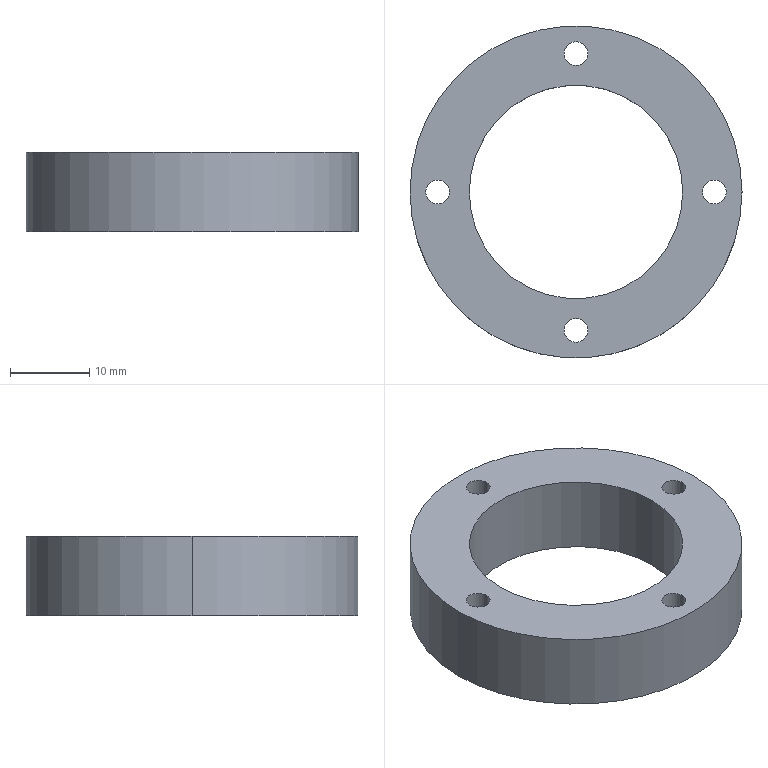Part | SolidWorks | features BaseBody 1 | 1 solid | 14 faces | box 42 x 42 x 10 mm | volume 7846 mm3 | cylinder 12 | plane 2 | commonest cylinder face diameters 3 x8 27 x2 42 x2
STEP:
#1=CARTESIAN_POINT('',(-16.,0.,10.));
#2=VERTEX_POINT('',#1);
#3=CARTESIAN_POINT('',(-19.,0.,10.));
#4=VERTEX_POINT('',#3);
#5=CARTESIAN_POINT('',(-17.5,0.,10.));
#6=DIRECTION('',(0.,0.,-1.));
#7=DIRECTION('',(-1.,0.,0.));
#8=AXIS2_PLACEMENT_3D('',#5,#6,#7);
#9=CIRCLE('',#8,1.5);
#10=EDGE_CURVE('',#2,#4,#9,.T.);
#11=ORIENTED_EDGE('',*,*,#10,.F.);
#12=CARTESIAN_POINT('',(-16.,0.,0.));
#13=VERTEX_POINT('',#12);
#14=CARTESIAN_POINT('',(-16.,0.,10.));
#15=DIRECTION('',(0.,0.,-1.));
#16=VECTOR('',#15,1000.);
#17=LINE('',#14,#16);
#18=EDGE_CURVE('',#2,#13,#17,.T.);
#19=ORIENTED_EDGE('',*,*,#18,.T.);
#20=CARTESIAN_POINT('',(-19.,0.,0.));
#21=VERTEX_POINT('',#20);
#22=CARTESIAN_POINT('',(-17.5,0.,0.));
#23=DIRECTION('',(0.,0.,-1.));
#24=DIRECTION('',(-1.,0.,0.));
#25=AXIS2_PLACEMENT_3D('',#22,#23,#24);
#26=CIRCLE('',#25,1.5);
#27=EDGE_CURVE('',#13,#21,#26,.T.);
#28=ORIENTED_EDGE('',*,*,#27,.T.);
#29=CARTESIAN_POINT('',(-19.,0.,10.));
#30=DIRECTION('',(0.,0.,-1.));
#31=VECTOR('',#30,1000.);
#32=LINE('',#29,#31);
#33=EDGE_CURVE('',#4,#21,#32,.T.);
#34=ORIENTED_EDGE('',*,*,#33,.F.);
#35=EDGE_LOOP('',(#11,#19,#28,#34));
#36=FACE_OUTER_BOUND('',#35,.T.);
#37=CARTESIAN_POINT('',(-17.5,0.,10.));
#38=DIRECTION('',(0.,0.,-1.));
#39=DIRECTION('',(-1.,0.,0.));
#40=AXIS2_PLACEMENT_3D('',#37,#38,#39);
#41=CYLINDRICAL_SURFACE('',#40,1.5);
#42=ADVANCED_FACE('',(#36),#41,.F.);
#43=CARTESIAN_POINT('',(1.5,-17.5,10.));
#44=VERTEX_POINT('',#43);
#45=CARTESIAN_POINT('',(-1.5,-17.5,10.));
#46=VERTEX_POINT('',#45);
#47=CARTESIAN_POINT('',(0.,-17.5,10.));
#48=DIRECTION('',(0.,0.,-1.));
#49=DIRECTION('',(-1.,0.,0.));
#50=AXIS2_PLACEMENT_3D('',#47,#48,#49);
#51=CIRCLE('',#50,1.5);
#52=EDGE_CURVE('',#44,#46,#51,.T.);
#53=ORIENTED_EDGE('',*,*,#52,.F.);
#54=CARTESIAN_POINT('',(1.5,-17.5,0.));
#55=VERTEX_POINT('',#54);
#56=CARTESIAN_POINT('',(1.5,-17.5,10.));
#57=DIRECTION('',(0.,0.,-1.));
#58=VECTOR('',#57,1000.);
#59=LINE('',#56,#58);
#60=EDGE_CURVE('',#44,#55,#59,.T.);
#61=ORIENTED_EDGE('',*,*,#60,.T.);
#62=CARTESIAN_POINT('',(-1.5,-17.5,0.));
#63=VERTEX_POINT('',#62);
#64=CARTESIAN_POINT('',(0.,-17.5,0.));
#65=DIRECTION('',(0.,0.,-1.));
#66=DIRECTION('',(-1.,0.,0.));
#67=AXIS2_PLACEMENT_3D('',#64,#65,#66);
#68=CIRCLE('',#67,1.5);
#69=EDGE_CURVE('',#55,#63,#68,.T.);
#70=ORIENTED_EDGE('',*,*,#69,.T.);
#71=CARTESIAN_POINT('',(-1.5,-17.5,10.));
#72=DIRECTION('',(0.,0.,-1.));
#73=VECTOR('',#72,1000.);
#74=LINE('',#71,#73);
#75=EDGE_CURVE('',#46,#63,#74,.T.);
#76=ORIENTED_EDGE('',*,*,#75,.F.);
#77=EDGE_LOOP('',(#53,#61,#70,#76));
#78=FACE_OUTER_BOUND('',#77,.T.);
#79=CARTESIAN_POINT('',(0.,-17.5,10.));
#80=DIRECTION('',(0.,0.,-1.));
#81=DIRECTION('',(-1.,0.,0.));
#82=AXIS2_PLACEMENT_3D('',#79,#80,#81);
#83=CYLINDRICAL_SURFACE('',#82,1.5);
#84=ADVANCED_FACE('',(#78),#83,.F.);
#85=CARTESIAN_POINT('',(19.,0.,10.));
#86=VERTEX_POINT('',#85);
#87=CARTESIAN_POINT('',(16.,0.,10.));
#88=VERTEX_POINT('',#87);
#89=CARTESIAN_POINT('',(17.5,0.,10.));
#90=DIRECTION('',(0.,0.,-1.));
#91=DIRECTION('',(-1.,0.,0.));
#92=AXIS2_PLACEMENT_3D('',#89,#90,#91);
#93=CIRCLE('',#92,1.5);
#94=EDGE_CURVE('',#86,#88,#93,.T.);
#95=ORIENTED_EDGE('',*,*,#94,.F.);
#96=CARTESIAN_POINT('',(19.,0.,0.));
#97=VERTEX_POINT('',#96);
#98=CARTESIAN_POINT('',(19.,0.,10.));
#99=DIRECTION('',(0.,0.,-1.));
#100=VECTOR('',#99,1000.);
#101=LINE('',#98,#100);
#102=EDGE_CURVE('',#86,#97,#101,.T.);
#103=ORIENTED_EDGE('',*,*,#102,.T.);
#104=CARTESIAN_POINT('',(16.,0.,0.));
#105=VERTEX_POINT('',#104);
#106=CARTESIAN_POINT('',(17.5,0.,0.));
#107=DIRECTION('',(0.,0.,-1.));
#108=DIRECTION('',(-1.,0.,0.));
#109=AXIS2_PLACEMENT_3D('',#106,#107,#108);
#110=CIRCLE('',#109,1.5);
#111=EDGE_CURVE('',#97,#105,#110,.T.);
#112=ORIENTED_EDGE('',*,*,#111,.T.);
#113=CARTESIAN_POINT('',(16.,0.,10.));
#114=DIRECTION('',(0.,0.,-1.));
#115=VECTOR('',#114,1000.);
#116=LINE('',#113,#115);
#117=EDGE_CURVE('',#88,#105,#116,.T.);
#118=ORIENTED_EDGE('',*,*,#117,.F.);
#119=EDGE_LOOP('',(#95,#103,#112,#118));
#120=FACE_OUTER_BOUND('',#119,.T.);
#121=CARTESIAN_POINT('',(17.5,0.,10.));
#122=DIRECTION('',(0.,0.,-1.));
#123=DIRECTION('',(-1.,0.,0.));
#124=AXIS2_PLACEMENT_3D('',#121,#122,#123);
#125=CYLINDRICAL_SURFACE('',#124,1.5);
#126=ADVANCED_FACE('',(#120),#125,.F.);
#127=CARTESIAN_POINT('',(1.5,17.5,10.));
#128=VERTEX_POINT('',#127);
#129=CARTESIAN_POINT('',(-1.5,17.5,10.));
#130=VERTEX_POINT('',#129);
#131=CARTESIAN_POINT('',(0.,17.5,10.));
#132=DIRECTION('',(0.,0.,-1.));
#133=DIRECTION('',(-1.,0.,0.));
#134=AXIS2_PLACEMENT_3D('',#131,#132,#133);
#135=CIRCLE('',#134,1.5);
#136=EDGE_CURVE('',#128,#130,#135,.T.);
#137=ORIENTED_EDGE('',*,*,#136,.F.);
#138=CARTESIAN_POINT('',(1.5,17.5,0.));
#139=VERTEX_POINT('',#138);
#140=CARTESIAN_POINT('',(1.5,17.5,10.));
#141=DIRECTION('',(0.,0.,-1.));
#142=VECTOR('',#141,1000.);
#143=LINE('',#140,#142);
#144=EDGE_CURVE('',#128,#139,#143,.T.);
#145=ORIENTED_EDGE('',*,*,#144,.T.);
#146=CARTESIAN_POINT('',(-1.5,17.5,0.));
#147=VERTEX_POINT('',#146);
#148=CARTESIAN_POINT('',(0.,17.5,0.));
#149=DIRECTION('',(0.,0.,-1.));
#150=DIRECTION('',(-1.,0.,0.));
#151=AXIS2_PLACEMENT_3D('',#148,#149,#150);
#152=CIRCLE('',#151,1.5);
#153=EDGE_CURVE('',#139,#147,#152,.T.);
#154=ORIENTED_EDGE('',*,*,#153,.T.);
#155=CARTESIAN_POINT('',(-1.5,17.5,10.));
#156=DIRECTION('',(0.,0.,-1.));
#157=VECTOR('',#156,1000.);
#158=LINE('',#155,#157);
#159=EDGE_CURVE('',#130,#147,#158,.T.);
#160=ORIENTED_EDGE('',*,*,#159,.F.);
#161=EDGE_LOOP('',(#137,#145,#154,#160));
#162=FACE_OUTER_BOUND('',#161,.T.);
#163=CARTESIAN_POINT('',(0.,17.5,10.));
#164=DIRECTION('',(0.,0.,-1.));
#165=DIRECTION('',(-1.,0.,0.));
#166=AXIS2_PLACEMENT_3D('',#163,#164,#165);
#167=CYLINDRICAL_SURFACE('',#166,1.5);
#168=ADVANCED_FACE('',(#162),#167,.F.);
#169=CARTESIAN_POINT('',(-21.,0.,10.));
#170=VERTEX_POINT('',#169);
#171=CARTESIAN_POINT('',(21.,0.,10.));
#172=VERTEX_POINT('',#171);
#173=CARTESIAN_POINT('',(0.,0.,10.));
#174=DIRECTION('',(0.,0.,-1.));
#175=DIRECTION('',(-1.,0.,0.));
#176=AXIS2_PLACEMENT_3D('',#173,#174,#175);
#177=CIRCLE('',#176,21.);
#178=EDGE_CURVE('',#170,#172,#177,.T.);
#179=ORIENTED_EDGE('',*,*,#178,.T.);
#180=CARTESIAN_POINT('',(21.,0.,0.));
#181=VERTEX_POINT('',#180);
#182=CARTESIAN_POINT('',(21.,0.,10.));
#183=DIRECTION('',(0.,0.,-1.));
#184=VECTOR('',#183,1000.);
#185=LINE('',#182,#184);
#186=EDGE_CURVE('',#172,#181,#185,.T.);
#187=ORIENTED_EDGE('',*,*,#186,.T.);
#188=CARTESIAN_POINT('',(-21.,0.,0.));
#189=VERTEX_POINT('',#188);
#190=CARTESIAN_POINT('',(0.,0.,0.));
#191=DIRECTION('',(0.,0.,1.));
#192=DIRECTION('',(-1.,0.,0.));
#193=AXIS2_PLACEMENT_3D('',#190,#191,#192);
#194=CIRCLE('',#193,21.);
#195=EDGE_CURVE('',#181,#189,#194,.T.);
#196=ORIENTED_EDGE('',*,*,#195,.T.);
#197=CARTESIAN_POINT('',(-21.,0.,10.));
#198=DIRECTION('',(0.,0.,-1.));
#199=VECTOR('',#198,1000.);
#200=LINE('',#197,#199);
#201=EDGE_CURVE('',#170,#189,#200,.T.);
#202=ORIENTED_EDGE('',*,*,#201,.F.);
#203=EDGE_LOOP('',(#179,#187,#196,#202));
#204=FACE_OUTER_BOUND('',#203,.T.);
#205=CARTESIAN_POINT('',(0.,0.,10.));
#206=DIRECTION('',(0.,0.,-1.));
#207=DIRECTION('',(-1.,0.,0.));
#208=AXIS2_PLACEMENT_3D('',#205,#206,#207);
#209=CYLINDRICAL_SURFACE('',#208,21.);
#210=ADVANCED_FACE('',(#204),#209,.T.);
#211=CARTESIAN_POINT('',(13.5,0.,0.));
#212=VERTEX_POINT('',#211);
#213=CARTESIAN_POINT('',(-13.5,0.,0.));
#214=VERTEX_POINT('',#213);
#215=CARTESIAN_POINT('',(0.,0.,0.));
#216=DIRECTION('',(0.,0.,-1.));
#217=DIRECTION('',(1.,0.,0.));
#218=AXIS2_PLACEMENT_3D('',#215,#216,#217);
#219=CIRCLE('',#218,13.5);
#220=EDGE_CURVE('',#212,#214,#219,.T.);
#221=ORIENTED_EDGE('',*,*,#220,.T.);
#222=CARTESIAN_POINT('',(-13.5,0.,10.));
#223=VERTEX_POINT('',#222);
#224=CARTESIAN_POINT('',(-13.5,0.,0.));
#225=DIRECTION('',(0.,0.,1.));
#226=VECTOR('',#225,1000.);
#227=LINE('',#224,#226);
#228=EDGE_CURVE('',#214,#223,#227,.T.);
#229=ORIENTED_EDGE('',*,*,#228,.T.);
#230=CARTESIAN_POINT('',(13.5,0.,10.));
#231=VERTEX_POINT('',#230);
#232=CARTESIAN_POINT('',(0.,0.,10.));
#233=DIRECTION('',(0.,0.,-1.));
#234=DIRECTION('',(1.,0.,0.));
#235=AXIS2_PLACEMENT_3D('',#232,#233,#234);
#236=CIRCLE('',#235,13.5);
#237=EDGE_CURVE('',#231,#223,#236,.T.);
#238=ORIENTED_EDGE('',*,*,#237,.F.);
#239=CARTESIAN_POINT('',(13.5,0.,0.));
#240=DIRECTION('',(0.,0.,1.));
#241=VECTOR('',#240,1000.);
#242=LINE('',#239,#241);
#243=EDGE_CURVE('',#212,#231,#242,.T.);
#244=ORIENTED_EDGE('',*,*,#243,.F.);
#245=EDGE_LOOP('',(#221,#229,#238,#244));
#246=FACE_OUTER_BOUND('',#245,.T.);
#247=CARTESIAN_POINT('',(0.,0.,0.));
#248=DIRECTION('',(0.,0.,1.));
#249=DIRECTION('',(1.,0.,0.));
#250=AXIS2_PLACEMENT_3D('',#247,#248,#249);
#251=CYLINDRICAL_SURFACE('',#250,13.5);
#252=ADVANCED_FACE('',(#246),#251,.F.);
#253=CARTESIAN_POINT('',(-17.5,0.,0.));
#254=DIRECTION('',(0.,0.,-1.));
#255=DIRECTION('',(-1.,0.,0.));
#256=AXIS2_PLACEMENT_3D('',#253,#254,#255);
#257=CIRCLE('',#256,1.5);
#258=EDGE_CURVE('',#21,#13,#257,.T.);
#259=ORIENTED_EDGE('',*,*,#258,.F.);
#260=ORIENTED_EDGE('',*,*,#27,.F.);
#261=EDGE_LOOP('',(#259,#260));
#262=FACE_BOUND('',#261,.T.);
#263=CARTESIAN_POINT('',(0.,-17.5,0.));
#264=DIRECTION('',(0.,0.,-1.));
#265=DIRECTION('',(-1.,0.,0.));
#266=AXIS2_PLACEMENT_3D('',#263,#264,#265);
#267=CIRCLE('',#266,1.5);
#268=EDGE_CURVE('',#63,#55,#267,.T.);
#269=ORIENTED_EDGE('',*,*,#268,.F.);
#270=ORIENTED_EDGE('',*,*,#69,.F.);
#271=EDGE_LOOP('',(#269,#270));
#272=FACE_BOUND('',#271,.T.);
#273=CARTESIAN_POINT('',(17.5,0.,0.));
#274=DIRECTION('',(0.,0.,-1.));
#275=DIRECTION('',(-1.,0.,0.));
#276=AXIS2_PLACEMENT_3D('',#273,#274,#275);
#277=CIRCLE('',#276,1.5);
#278=EDGE_CURVE('',#105,#97,#277,.T.);
#279=ORIENTED_EDGE('',*,*,#278,.F.);
#280=ORIENTED_EDGE('',*,*,#111,.F.);
#281=EDGE_LOOP('',(#279,#280));
#282=FACE_BOUND('',#281,.T.);
#283=CARTESIAN_POINT('',(0.,17.5,0.));
#284=DIRECTION('',(0.,0.,-1.));
#285=DIRECTION('',(-1.,0.,0.));
#286=AXIS2_PLACEMENT_3D('',#283,#284,#285);
#287=CIRCLE('',#286,1.5);
#288=EDGE_CURVE('',#147,#139,#287,.T.);
#289=ORIENTED_EDGE('',*,*,#288,.F.);
#290=ORIENTED_EDGE('',*,*,#153,.F.);
#291=EDGE_LOOP('',(#289,#290));
#292=FACE_BOUND('',#291,.T.);
#293=CARTESIAN_POINT('',(0.,0.,0.));
#294=DIRECTION('',(0.,0.,1.));
#295=DIRECTION('',(-1.,0.,0.));
#296=AXIS2_PLACEMENT_3D('',#293,#294,#295);
#297=CIRCLE('',#296,21.);
#298=EDGE_CURVE('',#189,#181,#297,.T.);
#299=ORIENTED_EDGE('',*,*,#298,.F.);
#300=ORIENTED_EDGE('',*,*,#195,.F.);
#301=EDGE_LOOP('',(#299,#300));
#302=FACE_OUTER_BOUND('',#301,.T.);
#303=ORIENTED_EDGE('',*,*,#220,.F.);
#304=CARTESIAN_POINT('',(0.,0.,0.));
#305=DIRECTION('',(0.,0.,-1.));
#306=DIRECTION('',(1.,0.,0.));
#307=AXIS2_PLACEMENT_3D('',#304,#305,#306);
#308=CIRCLE('',#307,13.5);
#309=EDGE_CURVE('',#214,#212,#308,.T.);
#310=ORIENTED_EDGE('',*,*,#309,.F.);
#311=EDGE_LOOP('',(#303,#310));
#312=FACE_BOUND('',#311,.T.);
#313=CARTESIAN_POINT('',(0.,0.,0.));
#314=DIRECTION('',(0.,0.,1.));
#315=DIRECTION('',(1.,0.,0.));
#316=AXIS2_PLACEMENT_3D('',#313,#314,#315);
#317=PLANE('',#316);
#318=ADVANCED_FACE('',(#262,#272,#282,#292,#302,#312),#317,.F.);
#319=ORIENTED_EDGE('',*,*,#18,.F.);
#320=CARTESIAN_POINT('',(-17.5,0.,10.));
#321=DIRECTION('',(0.,0.,-1.));
#322=DIRECTION('',(-1.,0.,0.));
#323=AXIS2_PLACEMENT_3D('',#320,#321,#322);
#324=CIRCLE('',#323,1.5);
#325=EDGE_CURVE('',#4,#2,#324,.T.);
#326=ORIENTED_EDGE('',*,*,#325,.F.);
#327=ORIENTED_EDGE('',*,*,#33,.T.);
#328=ORIENTED_EDGE('',*,*,#258,.T.);
#329=EDGE_LOOP('',(#319,#326,#327,#328));
#330=FACE_OUTER_BOUND('',#329,.T.);
#331=CARTESIAN_POINT('',(-17.5,0.,10.));
#332=DIRECTION('',(0.,0.,-1.));
#333=DIRECTION('',(-1.,0.,0.));
#334=AXIS2_PLACEMENT_3D('',#331,#332,#333);
#335=CYLINDRICAL_SURFACE('',#334,1.5);
#336=ADVANCED_FACE('',(#330),#335,.F.);
#337=ORIENTED_EDGE('',*,*,#60,.F.);
#338=CARTESIAN_POINT('',(0.,-17.5,10.));
#339=DIRECTION('',(0.,0.,-1.));
#340=DIRECTION('',(-1.,0.,0.));
#341=AXIS2_PLACEMENT_3D('',#338,#339,#340);
#342=CIRCLE('',#341,1.5);
#343=EDGE_CURVE('',#46,#44,#342,.T.);
#344=ORIENTED_EDGE('',*,*,#343,.F.);
#345=ORIENTED_EDGE('',*,*,#75,.T.);
#346=ORIENTED_EDGE('',*,*,#268,.T.);
#347=EDGE_LOOP('',(#337,#344,#345,#346));
#348=FACE_OUTER_BOUND('',#347,.T.);
#349=CARTESIAN_POINT('',(0.,-17.5,10.));
#350=DIRECTION('',(0.,0.,-1.));
#351=DIRECTION('',(-1.,0.,0.));
#352=AXIS2_PLACEMENT_3D('',#349,#350,#351);
#353=CYLINDRICAL_SURFACE('',#352,1.5);
#354=ADVANCED_FACE('',(#348),#353,.F.);
#355=ORIENTED_EDGE('',*,*,#102,.F.);
#356=CARTESIAN_POINT('',(17.5,0.,10.));
#357=DIRECTION('',(0.,0.,-1.));
#358=DIRECTION('',(-1.,0.,0.));
#359=AXIS2_PLACEMENT_3D('',#356,#357,#358);
#360=CIRCLE('',#359,1.5);
#361=EDGE_CURVE('',#88,#86,#360,.T.);
#362=ORIENTED_EDGE('',*,*,#361,.F.);
#363=ORIENTED_EDGE('',*,*,#117,.T.);
#364=ORIENTED_EDGE('',*,*,#278,.T.);
#365=EDGE_LOOP('',(#355,#362,#363,#364));
#366=FACE_OUTER_BOUND('',#365,.T.);
#367=CARTESIAN_POINT('',(17.5,0.,10.));
#368=DIRECTION('',(0.,0.,-1.));
#369=DIRECTION('',(-1.,0.,0.));
#370=AXIS2_PLACEMENT_3D('',#367,#368,#369);
#371=CYLINDRICAL_SURFACE('',#370,1.5);
#372=ADVANCED_FACE('',(#366),#371,.F.);
#373=ORIENTED_EDGE('',*,*,#144,.F.);
#374=CARTESIAN_POINT('',(0.,17.5,10.));
#375=DIRECTION('',(0.,0.,-1.));
#376=DIRECTION('',(-1.,0.,0.));
#377=AXIS2_PLACEMENT_3D('',#374,#375,#376);
#378=CIRCLE('',#377,1.5);
#379=EDGE_CURVE('',#130,#128,#378,.T.);
#380=ORIENTED_EDGE('',*,*,#379,.F.);
#381=ORIENTED_EDGE('',*,*,#159,.T.);
#382=ORIENTED_EDGE('',*,*,#288,.T.);
#383=EDGE_LOOP('',(#373,#380,#381,#382));
#384=FACE_OUTER_BOUND('',#383,.T.);
#385=CARTESIAN_POINT('',(0.,17.5,10.));
#386=DIRECTION('',(0.,0.,-1.));
#387=DIRECTION('',(-1.,0.,0.));
#388=AXIS2_PLACEMENT_3D('',#385,#386,#387);
#389=CYLINDRICAL_SURFACE('',#388,1.5);
#390=ADVANCED_FACE('',(#384),#389,.F.);
#391=ORIENTED_EDGE('',*,*,#186,.F.);
#392=CARTESIAN_POINT('',(0.,0.,10.));
#393=DIRECTION('',(0.,0.,-1.));
#394=DIRECTION('',(-1.,0.,0.));
#395=AXIS2_PLACEMENT_3D('',#392,#393,#394);
#396=CIRCLE('',#395,21.);
#397=EDGE_CURVE('',#172,#170,#396,.T.);
#398=ORIENTED_EDGE('',*,*,#397,.T.);
#399=ORIENTED_EDGE('',*,*,#201,.T.);
#400=ORIENTED_EDGE('',*,*,#298,.T.);
#401=EDGE_LOOP('',(#391,#398,#399,#400));
#402=FACE_OUTER_BOUND('',#401,.T.);
#403=CARTESIAN_POINT('',(0.,0.,10.));
#404=DIRECTION('',(0.,0.,-1.));
#405=DIRECTION('',(-1.,0.,0.));
#406=AXIS2_PLACEMENT_3D('',#403,#404,#405);
#407=CYLINDRICAL_SURFACE('',#406,21.);
#408=ADVANCED_FACE('',(#402),#407,.T.);
#409=ORIENTED_EDGE('',*,*,#228,.F.);
#410=ORIENTED_EDGE('',*,*,#309,.T.);
#411=ORIENTED_EDGE('',*,*,#243,.T.);
#412=CARTESIAN_POINT('',(0.,0.,10.));
#413=DIRECTION('',(0.,0.,-1.));
#414=DIRECTION('',(1.,0.,0.));
#415=AXIS2_PLACEMENT_3D('',#412,#413,#414);
#416=CIRCLE('',#415,13.5);
#417=EDGE_CURVE('',#223,#231,#416,.T.);
#418=ORIENTED_EDGE('',*,*,#417,.F.);
#419=EDGE_LOOP('',(#409,#410,#411,#418));
#420=FACE_OUTER_BOUND('',#419,.T.);
#421=CARTESIAN_POINT('',(0.,0.,0.));
#422=DIRECTION('',(0.,0.,1.));
#423=DIRECTION('',(1.,0.,0.));
#424=AXIS2_PLACEMENT_3D('',#421,#422,#423);
#425=CYLINDRICAL_SURFACE('',#424,13.5);
#426=ADVANCED_FACE('',(#420),#425,.F.);
#427=ORIENTED_EDGE('',*,*,#325,.T.);
#428=ORIENTED_EDGE('',*,*,#10,.T.);
#429=EDGE_LOOP('',(#427,#428));
#430=FACE_BOUND('',#429,.T.);
#431=ORIENTED_EDGE('',*,*,#361,.T.);
#432=ORIENTED_EDGE('',*,*,#94,.T.);
#433=EDGE_LOOP('',(#431,#432));
#434=FACE_BOUND('',#433,.T.);
#435=ORIENTED_EDGE('',*,*,#178,.F.);
#436=ORIENTED_EDGE('',*,*,#397,.F.);
#437=EDGE_LOOP('',(#435,#436));
#438=FACE_OUTER_BOUND('',#437,.T.);
#439=ORIENTED_EDGE('',*,*,#379,.T.);
#440=ORIENTED_EDGE('',*,*,#136,.T.);
#441=EDGE_LOOP('',(#439,#440));
#442=FACE_BOUND('',#441,.T.);
#443=ORIENTED_EDGE('',*,*,#343,.T.);
#444=ORIENTED_EDGE('',*,*,#52,.T.);
#445=EDGE_LOOP('',(#443,#444));
#446=FACE_BOUND('',#445,.T.);
#447=ORIENTED_EDGE('',*,*,#237,.T.);
#448=ORIENTED_EDGE('',*,*,#417,.T.);
#449=EDGE_LOOP('',(#447,#448));
#450=FACE_BOUND('',#449,.T.);
#451=CARTESIAN_POINT('',(0.,0.,10.));
#452=DIRECTION('',(0.,0.,1.));
#453=DIRECTION('',(1.,0.,0.));
#454=AXIS2_PLACEMENT_3D('',#451,#452,#453);
#455=PLANE('',#454);
#456=ADVANCED_FACE('',(#430,#434,#438,#442,#446,#450),#455,.T.);
#457=CLOSED_SHELL('',(#42,#84,#126,#168,#210,#252,#318,#336,#354,#372,#390,#408,#426,#456));
#458=MANIFOLD_SOLID_BREP('',#457);
#459=CARTESIAN_POINT('',(0.,0.,0.));
#460=DIRECTION('',(0.,0.,1.));
#461=DIRECTION('',(1.,0.,0.));
#462=AXIS2_PLACEMENT_3D('',#459,#460,#461);
#463=(LENGTH_UNIT()NAMED_UNIT(*)SI_UNIT(.MILLI.,.METRE.));
#464=UNCERTAINTY_MEASURE_WITH_UNIT(LENGTH_MEASURE(0.00001),#463,'','');
#465=(NAMED_UNIT(*)PLANE_ANGLE_UNIT()SI_UNIT($,.RADIAN.));
#466=(NAMED_UNIT(*)SI_UNIT($,.STERADIAN.)SOLID_ANGLE_UNIT());
#467=(GEOMETRIC_REPRESENTATION_CONTEXT(3)GLOBAL_UNCERTAINTY_ASSIGNED_CONTEXT((#464))GLOBAL_UNIT_ASSIGNED_CONTEXT((#463,#465,#466))REPRESENTATION_CONTEXT('',''));
#468=ADVANCED_BREP_SHAPE_REPRESENTATION('',(#458,#462),#467);